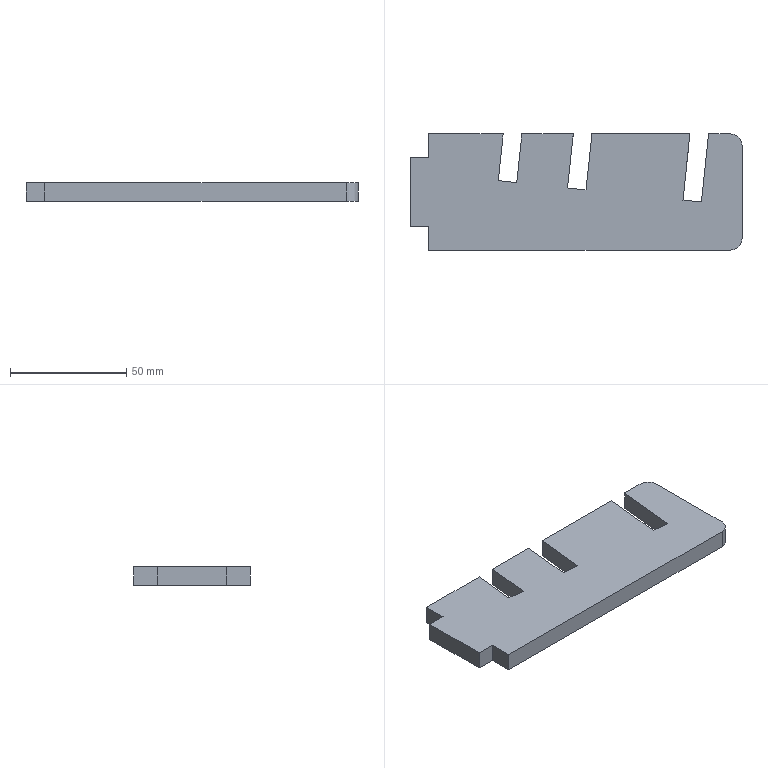Part | SolidWorks | features Fillet 1, FlatPattern 1, SMBaseFlange 1, SheetMetal 1 | 1 solid | 24 faces | box 143 x 50 x 8 mm | volume 51129 mm3 | plane 22 | cylinder 2 | commonest cylinder face diameters 10 x2
STEP:
#1=CARTESIAN_POINT('',(690.834,-177.819,0.));
#2=VERTEX_POINT('',#1);
#3=CARTESIAN_POINT('',(693.823,-149.341,0.));
#4=VERTEX_POINT('',#3);
#5=CARTESIAN_POINT('',(693.823,-149.341,0.));
#6=DIRECTION('',(0.1044,0.9945,0.));
#7=VECTOR('',#6,1000.);
#8=LINE('',#5,#7);
#9=EDGE_CURVE('',#2,#4,#8,.T.);
#10=ORIENTED_EDGE('',*,*,#9,.F.);
#11=CARTESIAN_POINT('',(690.834,-177.819,-8.));
#12=VERTEX_POINT('',#11);
#13=CARTESIAN_POINT('',(690.834,-177.819,-8.));
#14=DIRECTION('',(0.,0.,1.));
#15=VECTOR('',#14,1000.);
#16=LINE('',#13,#15);
#17=EDGE_CURVE('',#12,#2,#16,.T.);
#18=ORIENTED_EDGE('',*,*,#17,.F.);
#19=CARTESIAN_POINT('',(693.823,-149.341,-8.));
#20=VERTEX_POINT('',#19);
#21=CARTESIAN_POINT('',(693.823,-149.341,-8.));
#22=DIRECTION('',(0.1044,0.9945,0.));
#23=VECTOR('',#22,1000.);
#24=LINE('',#21,#23);
#25=EDGE_CURVE('',#12,#20,#24,.T.);
#26=ORIENTED_EDGE('',*,*,#25,.T.);
#27=CARTESIAN_POINT('',(693.823,-149.341,-8.));
#28=DIRECTION('',(0.,0.,1.));
#29=VECTOR('',#28,1000.);
#30=LINE('',#27,#29);
#31=EDGE_CURVE('',#20,#4,#30,.T.);
#32=ORIENTED_EDGE('',*,*,#31,.T.);
#33=EDGE_LOOP('',(#10,#18,#26,#32));
#34=FACE_OUTER_BOUND('',#33,.T.);
#35=CARTESIAN_POINT('',(693.823,-149.341,-8.));
#36=DIRECTION('',(0.9945,-0.1044,0.));
#37=DIRECTION('',(0.1044,0.9945,0.));
#38=AXIS2_PLACEMENT_3D('',#35,#36,#37);
#39=PLANE('',#38);
#40=ADVANCED_FACE('',(#34),#39,.T.);
#41=CARTESIAN_POINT('',(698.79,-178.654,0.));
#42=VERTEX_POINT('',#41);
#43=CARTESIAN_POINT('',(690.834,-177.819,0.));
#44=DIRECTION('',(-0.9945,0.1044,0.));
#45=VECTOR('',#44,1000.);
#46=LINE('',#43,#45);
#47=EDGE_CURVE('',#42,#2,#46,.T.);
#48=ORIENTED_EDGE('',*,*,#47,.F.);
#49=CARTESIAN_POINT('',(698.79,-178.654,-8.));
#50=VERTEX_POINT('',#49);
#51=CARTESIAN_POINT('',(698.79,-178.654,-8.));
#52=DIRECTION('',(0.,0.,1.));
#53=VECTOR('',#52,1000.);
#54=LINE('',#51,#53);
#55=EDGE_CURVE('',#50,#42,#54,.T.);
#56=ORIENTED_EDGE('',*,*,#55,.F.);
#57=CARTESIAN_POINT('',(690.834,-177.819,-8.));
#58=DIRECTION('',(-0.9945,0.1044,0.));
#59=VECTOR('',#58,1000.);
#60=LINE('',#57,#59);
#61=EDGE_CURVE('',#50,#12,#60,.T.);
#62=ORIENTED_EDGE('',*,*,#61,.T.);
#63=ORIENTED_EDGE('',*,*,#17,.T.);
#64=EDGE_LOOP('',(#48,#56,#62,#63));
#65=FACE_OUTER_BOUND('',#64,.T.);
#66=CARTESIAN_POINT('',(690.834,-177.819,-8.));
#67=DIRECTION('',(0.1044,0.9945,0.));
#68=DIRECTION('',(-0.9945,0.1044,0.));
#69=AXIS2_PLACEMENT_3D('',#66,#67,#68);
#70=PLANE('',#69);
#71=ADVANCED_FACE('',(#65),#70,.T.);
#72=CARTESIAN_POINT('',(701.867,-149.341,0.));
#73=VERTEX_POINT('',#72);
#74=CARTESIAN_POINT('',(698.79,-178.654,0.));
#75=DIRECTION('',(-0.1044,-0.9945,0.));
#76=VECTOR('',#75,1000.);
#77=LINE('',#74,#76);
#78=EDGE_CURVE('',#73,#42,#77,.T.);
#79=ORIENTED_EDGE('',*,*,#78,.F.);
#80=CARTESIAN_POINT('',(701.867,-149.341,-8.));
#81=VERTEX_POINT('',#80);
#82=CARTESIAN_POINT('',(701.867,-149.341,-8.));
#83=DIRECTION('',(0.,0.,1.));
#84=VECTOR('',#83,1000.);
#85=LINE('',#82,#84);
#86=EDGE_CURVE('',#81,#73,#85,.T.);
#87=ORIENTED_EDGE('',*,*,#86,.F.);
#88=CARTESIAN_POINT('',(698.79,-178.654,-8.));
#89=DIRECTION('',(-0.1044,-0.9945,0.));
#90=VECTOR('',#89,1000.);
#91=LINE('',#88,#90);
#92=EDGE_CURVE('',#81,#50,#91,.T.);
#93=ORIENTED_EDGE('',*,*,#92,.T.);
#94=ORIENTED_EDGE('',*,*,#55,.T.);
#95=EDGE_LOOP('',(#79,#87,#93,#94));
#96=FACE_OUTER_BOUND('',#95,.T.);
#97=CARTESIAN_POINT('',(698.79,-178.654,-8.));
#98=DIRECTION('',(-0.9945,0.1044,0.));
#99=DIRECTION('',(-0.1044,-0.9945,0.));
#100=AXIS2_PLACEMENT_3D('',#97,#98,#99);
#101=PLANE('',#100);
#102=ADVANCED_FACE('',(#96),#101,.T.);
#103=CARTESIAN_POINT('',(711.248,-149.341,0.));
#104=VERTEX_POINT('',#103);
#105=CARTESIAN_POINT('',(701.867,-149.341,0.));
#106=DIRECTION('',(-1.,0.,0.));
#107=VECTOR('',#106,1000.);
#108=LINE('',#105,#107);
#109=EDGE_CURVE('',#104,#73,#108,.T.);
#110=ORIENTED_EDGE('',*,*,#109,.F.);
#111=CARTESIAN_POINT('',(711.248,-149.341,-8.));
#112=VERTEX_POINT('',#111);
#113=CARTESIAN_POINT('',(711.248,-149.341,-8.));
#114=DIRECTION('',(0.,0.,-1.));
#115=VECTOR('',#114,1000.);
#116=LINE('',#113,#115);
#117=EDGE_CURVE('',#104,#112,#116,.T.);
#118=ORIENTED_EDGE('',*,*,#117,.T.);
#119=CARTESIAN_POINT('',(701.867,-149.341,-8.));
#120=DIRECTION('',(-1.,0.,0.));
#121=VECTOR('',#120,1000.);
#122=LINE('',#119,#121);
#123=EDGE_CURVE('',#112,#81,#122,.T.);
#124=ORIENTED_EDGE('',*,*,#123,.T.);
#125=ORIENTED_EDGE('',*,*,#86,.T.);
#126=EDGE_LOOP('',(#110,#118,#124,#125));
#127=FACE_OUTER_BOUND('',#126,.T.);
#128=CARTESIAN_POINT('',(701.867,-149.341,-8.));
#129=DIRECTION('',(0.,1.,0.));
#130=DIRECTION('',(0.,0.,1.));
#131=AXIS2_PLACEMENT_3D('',#128,#129,#130);
#132=PLANE('',#131);
#133=ADVANCED_FACE('',(#127),#132,.T.);
#134=CARTESIAN_POINT('',(716.248,-194.341,-8.));
#135=VERTEX_POINT('',#134);
#136=CARTESIAN_POINT('',(716.248,-154.341,-8.));
#137=VERTEX_POINT('',#136);
#138=CARTESIAN_POINT('',(716.248,-149.341,-8.));
#139=DIRECTION('',(0.,1.,0.));
#140=VECTOR('',#139,1000.);
#141=LINE('',#138,#140);
#142=EDGE_CURVE('',#135,#137,#141,.T.);
#143=ORIENTED_EDGE('',*,*,#142,.T.);
#144=CARTESIAN_POINT('',(716.248,-154.341,0.));
#145=VERTEX_POINT('',#144);
#146=CARTESIAN_POINT('',(716.248,-154.341,-8.));
#147=DIRECTION('',(0.,0.,1.));
#148=VECTOR('',#147,1000.);
#149=LINE('',#146,#148);
#150=EDGE_CURVE('',#137,#145,#149,.T.);
#151=ORIENTED_EDGE('',*,*,#150,.T.);
#152=CARTESIAN_POINT('',(716.248,-194.341,0.));
#153=VERTEX_POINT('',#152);
#154=CARTESIAN_POINT('',(716.248,-149.341,0.));
#155=DIRECTION('',(0.,1.,0.));
#156=VECTOR('',#155,1000.);
#157=LINE('',#154,#156);
#158=EDGE_CURVE('',#153,#145,#157,.T.);
#159=ORIENTED_EDGE('',*,*,#158,.F.);
#160=CARTESIAN_POINT('',(716.248,-194.341,-8.));
#161=DIRECTION('',(0.,0.,-1.));
#162=VECTOR('',#161,1000.);
#163=LINE('',#160,#162);
#164=EDGE_CURVE('',#153,#135,#163,.T.);
#165=ORIENTED_EDGE('',*,*,#164,.T.);
#166=EDGE_LOOP('',(#143,#151,#159,#165));
#167=FACE_OUTER_BOUND('',#166,.T.);
#168=CARTESIAN_POINT('',(716.248,-149.341,-8.));
#169=DIRECTION('',(1.,0.,0.));
#170=DIRECTION('',(0.,0.,-1.));
#171=AXIS2_PLACEMENT_3D('',#168,#169,#170);
#172=PLANE('',#171);
#173=ADVANCED_FACE('',(#167),#172,.T.);
#174=CARTESIAN_POINT('',(581.248,-199.341,-8.));
#175=VERTEX_POINT('',#174);
#176=CARTESIAN_POINT('',(711.248,-199.341,-8.));
#177=VERTEX_POINT('',#176);
#178=CARTESIAN_POINT('',(581.248,-199.341,-8.));
#179=DIRECTION('',(1.,0.,0.));
#180=VECTOR('',#179,1000.);
#181=LINE('',#178,#180);
#182=EDGE_CURVE('',#175,#177,#181,.T.);
#183=ORIENTED_EDGE('',*,*,#182,.T.);
#184=CARTESIAN_POINT('',(711.248,-199.341,0.));
#185=VERTEX_POINT('',#184);
#186=CARTESIAN_POINT('',(711.248,-199.341,-8.));
#187=DIRECTION('',(0.,0.,1.));
#188=VECTOR('',#187,1000.);
#189=LINE('',#186,#188);
#190=EDGE_CURVE('',#177,#185,#189,.T.);
#191=ORIENTED_EDGE('',*,*,#190,.T.);
#192=CARTESIAN_POINT('',(581.248,-199.341,0.));
#193=VERTEX_POINT('',#192);
#194=CARTESIAN_POINT('',(581.248,-199.341,0.));
#195=DIRECTION('',(1.,0.,0.));
#196=VECTOR('',#195,1000.);
#197=LINE('',#194,#196);
#198=EDGE_CURVE('',#193,#185,#197,.T.);
#199=ORIENTED_EDGE('',*,*,#198,.F.);
#200=CARTESIAN_POINT('',(581.248,-199.341,-8.));
#201=DIRECTION('',(0.,0.,1.));
#202=VECTOR('',#201,1000.);
#203=LINE('',#200,#202);
#204=EDGE_CURVE('',#175,#193,#203,.T.);
#205=ORIENTED_EDGE('',*,*,#204,.F.);
#206=EDGE_LOOP('',(#183,#191,#199,#205));
#207=FACE_OUTER_BOUND('',#206,.T.);
#208=CARTESIAN_POINT('',(581.248,-199.341,-8.));
#209=DIRECTION('',(0.,-1.,0.));
#210=DIRECTION('',(0.,0.,-1.));
#211=AXIS2_PLACEMENT_3D('',#208,#209,#210);
#212=PLANE('',#211);
#213=ADVANCED_FACE('',(#207),#212,.T.);
#214=CARTESIAN_POINT('',(581.248,-189.341,0.));
#215=VERTEX_POINT('',#214);
#216=CARTESIAN_POINT('',(581.248,-189.341,0.));
#217=DIRECTION('',(0.,-1.,0.));
#218=VECTOR('',#217,1000.);
#219=LINE('',#216,#218);
#220=EDGE_CURVE('',#215,#193,#219,.T.);
#221=ORIENTED_EDGE('',*,*,#220,.F.);
#222=CARTESIAN_POINT('',(581.248,-189.341,-8.));
#223=VERTEX_POINT('',#222);
#224=CARTESIAN_POINT('',(581.248,-189.341,-8.));
#225=DIRECTION('',(0.,0.,1.));
#226=VECTOR('',#225,1000.);
#227=LINE('',#224,#226);
#228=EDGE_CURVE('',#223,#215,#227,.T.);
#229=ORIENTED_EDGE('',*,*,#228,.F.);
#230=CARTESIAN_POINT('',(581.248,-189.341,-8.));
#231=DIRECTION('',(0.,-1.,0.));
#232=VECTOR('',#231,1000.);
#233=LINE('',#230,#232);
#234=EDGE_CURVE('',#223,#175,#233,.T.);
#235=ORIENTED_EDGE('',*,*,#234,.T.);
#236=ORIENTED_EDGE('',*,*,#204,.T.);
#237=EDGE_LOOP('',(#221,#229,#235,#236));
#238=FACE_OUTER_BOUND('',#237,.T.);
#239=CARTESIAN_POINT('',(581.248,-189.341,-8.));
#240=DIRECTION('',(-1.,0.,0.));
#241=DIRECTION('',(0.,0.,1.));
#242=AXIS2_PLACEMENT_3D('',#239,#240,#241);
#243=PLANE('',#242);
#244=ADVANCED_FACE('',(#238),#243,.T.);
#245=CARTESIAN_POINT('',(573.248,-189.341,0.));
#246=VERTEX_POINT('',#245);
#247=CARTESIAN_POINT('',(573.248,-189.341,0.));
#248=DIRECTION('',(1.,0.,0.));
#249=VECTOR('',#248,1000.);
#250=LINE('',#247,#249);
#251=EDGE_CURVE('',#246,#215,#250,.T.);
#252=ORIENTED_EDGE('',*,*,#251,.F.);
#253=CARTESIAN_POINT('',(573.248,-189.341,-8.));
#254=VERTEX_POINT('',#253);
#255=CARTESIAN_POINT('',(573.248,-189.341,-8.));
#256=DIRECTION('',(0.,0.,1.));
#257=VECTOR('',#256,1000.);
#258=LINE('',#255,#257);
#259=EDGE_CURVE('',#254,#246,#258,.T.);
#260=ORIENTED_EDGE('',*,*,#259,.F.);
#261=CARTESIAN_POINT('',(573.248,-189.341,-8.));
#262=DIRECTION('',(1.,0.,0.));
#263=VECTOR('',#262,1000.);
#264=LINE('',#261,#263);
#265=EDGE_CURVE('',#254,#223,#264,.T.);
#266=ORIENTED_EDGE('',*,*,#265,.T.);
#267=ORIENTED_EDGE('',*,*,#228,.T.);
#268=EDGE_LOOP('',(#252,#260,#266,#267));
#269=FACE_OUTER_BOUND('',#268,.T.);
#270=CARTESIAN_POINT('',(573.248,-189.341,-8.));
#271=DIRECTION('',(0.,-1.,0.));
#272=DIRECTION('',(0.,0.,-1.));
#273=AXIS2_PLACEMENT_3D('',#270,#271,#272);
#274=PLANE('',#273);
#275=ADVANCED_FACE('',(#269),#274,.T.);
#276=CARTESIAN_POINT('',(573.248,-159.341,0.));
#277=VERTEX_POINT('',#276);
#278=CARTESIAN_POINT('',(573.248,-159.341,0.));
#279=DIRECTION('',(0.,-1.,0.));
#280=VECTOR('',#279,1000.);
#281=LINE('',#278,#280);
#282=EDGE_CURVE('',#277,#246,#281,.T.);
#283=ORIENTED_EDGE('',*,*,#282,.F.);
#284=CARTESIAN_POINT('',(573.248,-159.341,-8.));
#285=VERTEX_POINT('',#284);
#286=CARTESIAN_POINT('',(573.248,-159.341,-8.));
#287=DIRECTION('',(0.,0.,1.));
#288=VECTOR('',#287,1000.);
#289=LINE('',#286,#288);
#290=EDGE_CURVE('',#285,#277,#289,.T.);
#291=ORIENTED_EDGE('',*,*,#290,.F.);
#292=CARTESIAN_POINT('',(573.248,-159.341,-8.));
#293=DIRECTION('',(0.,-1.,0.));
#294=VECTOR('',#293,1000.);
#295=LINE('',#292,#294);
#296=EDGE_CURVE('',#285,#254,#295,.T.);
#297=ORIENTED_EDGE('',*,*,#296,.T.);
#298=ORIENTED_EDGE('',*,*,#259,.T.);
#299=EDGE_LOOP('',(#283,#291,#297,#298));
#300=FACE_OUTER_BOUND('',#299,.T.);
#301=CARTESIAN_POINT('',(573.248,-159.341,-8.));
#302=DIRECTION('',(-1.,0.,0.));
#303=DIRECTION('',(0.,0.,1.));
#304=AXIS2_PLACEMENT_3D('',#301,#302,#303);
#305=PLANE('',#304);
#306=ADVANCED_FACE('',(#300),#305,.T.);
#307=CARTESIAN_POINT('',(581.248,-159.341,0.));
#308=VERTEX_POINT('',#307);
#309=CARTESIAN_POINT('',(581.248,-159.341,0.));
#310=DIRECTION('',(-1.,0.,0.));
#311=VECTOR('',#310,1000.);
#312=LINE('',#309,#311);
#313=EDGE_CURVE('',#308,#277,#312,.T.);
#314=ORIENTED_EDGE('',*,*,#313,.F.);
#315=CARTESIAN_POINT('',(581.248,-159.341,-8.));
#316=VERTEX_POINT('',#315);
#317=CARTESIAN_POINT('',(581.248,-159.341,-8.));
#318=DIRECTION('',(0.,0.,1.));
#319=VECTOR('',#318,1000.);
#320=LINE('',#317,#319);
#321=EDGE_CURVE('',#316,#308,#320,.T.);
#322=ORIENTED_EDGE('',*,*,#321,.F.);
#323=CARTESIAN_POINT('',(581.248,-159.341,-8.));
#324=DIRECTION('',(-1.,0.,0.));
#325=VECTOR('',#324,1000.);
#326=LINE('',#323,#325);
#327=EDGE_CURVE('',#316,#285,#326,.T.);
#328=ORIENTED_EDGE('',*,*,#327,.T.);
#329=ORIENTED_EDGE('',*,*,#290,.T.);
#330=EDGE_LOOP('',(#314,#322,#328,#329));
#331=FACE_OUTER_BOUND('',#330,.T.);
#332=CARTESIAN_POINT('',(581.248,-159.341,-8.));
#333=DIRECTION('',(0.,1.,0.));
#334=DIRECTION('',(0.,0.,1.));
#335=AXIS2_PLACEMENT_3D('',#332,#333,#334);
#336=PLANE('',#335);
#337=ADVANCED_FACE('',(#331),#336,.T.);
#338=CARTESIAN_POINT('',(581.248,-149.341,0.));
#339=VERTEX_POINT('',#338);
#340=CARTESIAN_POINT('',(581.248,-149.341,0.));
#341=DIRECTION('',(0.,-1.,0.));
#342=VECTOR('',#341,1000.);
#343=LINE('',#340,#342);
#344=EDGE_CURVE('',#339,#308,#343,.T.);
#345=ORIENTED_EDGE('',*,*,#344,.F.);
#346=CARTESIAN_POINT('',(581.248,-149.341,-8.));
#347=VERTEX_POINT('',#346);
#348=CARTESIAN_POINT('',(581.248,-149.341,-8.));
#349=DIRECTION('',(0.,0.,1.));
#350=VECTOR('',#349,1000.);
#351=LINE('',#348,#350);
#352=EDGE_CURVE('',#347,#339,#351,.T.);
#353=ORIENTED_EDGE('',*,*,#352,.F.);
#354=CARTESIAN_POINT('',(581.248,-149.341,-8.));
#355=DIRECTION('',(0.,-1.,0.));
#356=VECTOR('',#355,1000.);
#357=LINE('',#354,#356);
#358=EDGE_CURVE('',#347,#316,#357,.T.);
#359=ORIENTED_EDGE('',*,*,#358,.T.);
#360=ORIENTED_EDGE('',*,*,#321,.T.);
#361=EDGE_LOOP('',(#345,#353,#359,#360));
#362=FACE_OUTER_BOUND('',#361,.T.);
#363=CARTESIAN_POINT('',(581.248,-149.341,-8.));
#364=DIRECTION('',(-1.,0.,0.));
#365=DIRECTION('',(0.,0.,1.));
#366=AXIS2_PLACEMENT_3D('',#363,#364,#365);
#367=PLANE('',#366);
#368=ADVANCED_FACE('',(#362),#367,.T.);
#369=CARTESIAN_POINT('',(613.384,-149.341,0.));
#370=VERTEX_POINT('',#369);
#371=CARTESIAN_POINT('',(581.248,-149.341,0.));
#372=DIRECTION('',(-1.,0.,0.));
#373=VECTOR('',#372,1000.);
#374=LINE('',#371,#373);
#375=EDGE_CURVE('',#370,#339,#374,.T.);
#376=ORIENTED_EDGE('',*,*,#375,.F.);
#377=CARTESIAN_POINT('',(613.384,-149.341,-8.));
#378=VERTEX_POINT('',#377);
#379=CARTESIAN_POINT('',(613.384,-149.341,-8.));
#380=DIRECTION('',(0.,0.,1.));
#381=VECTOR('',#380,1000.);
#382=LINE('',#379,#381);
#383=EDGE_CURVE('',#378,#370,#382,.T.);
#384=ORIENTED_EDGE('',*,*,#383,.F.);
#385=CARTESIAN_POINT('',(581.248,-149.341,-8.));
#386=DIRECTION('',(-1.,0.,0.));
#387=VECTOR('',#386,1000.);
#388=LINE('',#385,#387);
#389=EDGE_CURVE('',#378,#347,#388,.T.);
#390=ORIENTED_EDGE('',*,*,#389,.T.);
#391=ORIENTED_EDGE('',*,*,#352,.T.);
#392=EDGE_LOOP('',(#376,#384,#390,#391));
#393=FACE_OUTER_BOUND('',#392,.T.);
#394=CARTESIAN_POINT('',(581.248,-149.341,-8.));
#395=DIRECTION('',(0.,1.,0.));
#396=DIRECTION('',(0.,0.,1.));
#397=AXIS2_PLACEMENT_3D('',#394,#395,#396);
#398=PLANE('',#397);
#399=ADVANCED_FACE('',(#393),#398,.T.);
#400=CARTESIAN_POINT('',(611.271,-169.465,0.));
#401=VERTEX_POINT('',#400);
#402=CARTESIAN_POINT('',(611.271,-169.465,0.));
#403=DIRECTION('',(0.1044,0.9945,0.));
#404=VECTOR('',#403,1000.);
#405=LINE('',#402,#404);
#406=EDGE_CURVE('',#401,#370,#405,.T.);
#407=ORIENTED_EDGE('',*,*,#406,.F.);
#408=CARTESIAN_POINT('',(611.271,-169.465,-8.));
#409=VERTEX_POINT('',#408);
#410=CARTESIAN_POINT('',(611.271,-169.465,-8.));
#411=DIRECTION('',(0.,0.,1.));
#412=VECTOR('',#411,1000.);
#413=LINE('',#410,#412);
#414=EDGE_CURVE('',#409,#401,#413,.T.);
#415=ORIENTED_EDGE('',*,*,#414,.F.);
#416=CARTESIAN_POINT('',(611.271,-169.465,-8.));
#417=DIRECTION('',(0.1044,0.9945,0.));
#418=VECTOR('',#417,1000.);
#419=LINE('',#416,#418);
#420=EDGE_CURVE('',#409,#378,#419,.T.);
#421=ORIENTED_EDGE('',*,*,#420,.T.);
#422=ORIENTED_EDGE('',*,*,#383,.T.);
#423=EDGE_LOOP('',(#407,#415,#421,#422));
#424=FACE_OUTER_BOUND('',#423,.T.);
#425=CARTESIAN_POINT('',(611.271,-169.465,-8.));
#426=DIRECTION('',(0.9945,-0.1044,0.));
#427=DIRECTION('',(0.1044,0.9945,0.));
#428=AXIS2_PLACEMENT_3D('',#425,#426,#427);
#429=PLANE('',#428);
#430=ADVANCED_FACE('',(#424),#429,.T.);
#431=CARTESIAN_POINT('',(619.227,-170.301,0.));
#432=VERTEX_POINT('',#431);
#433=CARTESIAN_POINT('',(611.271,-169.465,0.));
#434=DIRECTION('',(-0.9945,0.1044,0.));
#435=VECTOR('',#434,1000.);
#436=LINE('',#433,#435);
#437=EDGE_CURVE('',#432,#401,#436,.T.);
#438=ORIENTED_EDGE('',*,*,#437,.F.);
#439=CARTESIAN_POINT('',(619.227,-170.301,-8.));
#440=VERTEX_POINT('',#439);
#441=CARTESIAN_POINT('',(619.227,-170.301,-8.));
#442=DIRECTION('',(0.,0.,1.));
#443=VECTOR('',#442,1000.);
#444=LINE('',#441,#443);
#445=EDGE_CURVE('',#440,#432,#444,.T.);
#446=ORIENTED_EDGE('',*,*,#445,.F.);
#447=CARTESIAN_POINT('',(611.271,-169.465,-8.));
#448=DIRECTION('',(-0.9945,0.1044,0.));
#449=VECTOR('',#448,1000.);
#450=LINE('',#447,#449);
#451=EDGE_CURVE('',#440,#409,#450,.T.);
#452=ORIENTED_EDGE('',*,*,#451,.T.);
#453=ORIENTED_EDGE('',*,*,#414,.T.);
#454=EDGE_LOOP('',(#438,#446,#452,#453));
#455=FACE_OUTER_BOUND('',#454,.T.);
#456=CARTESIAN_POINT('',(611.271,-169.465,-8.));
#457=DIRECTION('',(0.1044,0.9945,0.));
#458=DIRECTION('',(-0.9945,0.1044,0.));
#459=AXIS2_PLACEMENT_3D('',#456,#457,#458);
#460=PLANE('',#459);
#461=ADVANCED_FACE('',(#455),#460,.T.);
#462=CARTESIAN_POINT('',(621.428,-149.341,0.));
#463=VERTEX_POINT('',#462);
#464=CARTESIAN_POINT('',(619.227,-170.301,0.));
#465=DIRECTION('',(-0.1044,-0.9945,0.));
#466=VECTOR('',#465,1000.);
#467=LINE('',#464,#466);
#468=EDGE_CURVE('',#463,#432,#467,.T.);
#469=ORIENTED_EDGE('',*,*,#468,.F.);
#470=CARTESIAN_POINT('',(621.428,-149.341,-8.));
#471=VERTEX_POINT('',#470);
#472=CARTESIAN_POINT('',(621.428,-149.341,-8.));
#473=DIRECTION('',(0.,0.,1.));
#474=VECTOR('',#473,1000.);
#475=LINE('',#472,#474);
#476=EDGE_CURVE('',#471,#463,#475,.T.);
#477=ORIENTED_EDGE('',*,*,#476,.F.);
#478=CARTESIAN_POINT('',(619.227,-170.301,-8.));
#479=DIRECTION('',(-0.1044,-0.9945,0.));
#480=VECTOR('',#479,1000.);
#481=LINE('',#478,#480);
#482=EDGE_CURVE('',#471,#440,#481,.T.);
#483=ORIENTED_EDGE('',*,*,#482,.T.);
#484=ORIENTED_EDGE('',*,*,#445,.T.);
#485=EDGE_LOOP('',(#469,#477,#483,#484));
#486=FACE_OUTER_BOUND('',#485,.T.);
#487=CARTESIAN_POINT('',(619.227,-170.301,-8.));
#488=DIRECTION('',(-0.9945,0.1044,0.));
#489=DIRECTION('',(-0.1044,-0.9945,0.));
#490=AXIS2_PLACEMENT_3D('',#487,#488,#489);
#491=PLANE('',#490);
#492=ADVANCED_FACE('',(#486),#491,.T.);
#493=CARTESIAN_POINT('',(643.549,-149.341,0.));
#494=VERTEX_POINT('',#493);
#495=CARTESIAN_POINT('',(621.428,-149.341,0.));
#496=DIRECTION('',(-1.,0.,0.));
#497=VECTOR('',#496,1000.);
#498=LINE('',#495,#497);
#499=EDGE_CURVE('',#494,#463,#498,.T.);
#500=ORIENTED_EDGE('',*,*,#499,.F.);
#501=CARTESIAN_POINT('',(643.549,-149.341,-8.));
#502=VERTEX_POINT('',#501);
#503=CARTESIAN_POINT('',(643.549,-149.341,-8.));
#504=DIRECTION('',(0.,0.,1.));
#505=VECTOR('',#504,1000.);
#506=LINE('',#503,#505);
#507=EDGE_CURVE('',#502,#494,#506,.T.);
#508=ORIENTED_EDGE('',*,*,#507,.F.);
#509=CARTESIAN_POINT('',(621.428,-149.341,-8.));
#510=DIRECTION('',(-1.,0.,0.));
#511=VECTOR('',#510,1000.);
#512=LINE('',#509,#511);
#513=EDGE_CURVE('',#502,#471,#512,.T.);
#514=ORIENTED_EDGE('',*,*,#513,.T.);
#515=ORIENTED_EDGE('',*,*,#476,.T.);
#516=EDGE_LOOP('',(#500,#508,#514,#515));
#517=FACE_OUTER_BOUND('',#516,.T.);
#518=CARTESIAN_POINT('',(621.428,-149.341,-8.));
#519=DIRECTION('',(0.,1.,0.));
#520=DIRECTION('',(0.,0.,1.));
#521=AXIS2_PLACEMENT_3D('',#518,#519,#520);
#522=PLANE('',#521);
#523=ADVANCED_FACE('',(#517),#522,.T.);
#524=CARTESIAN_POINT('',(641.107,-172.598,0.));
#525=VERTEX_POINT('',#524);
#526=CARTESIAN_POINT('',(641.107,-172.598,0.));
#527=DIRECTION('',(0.1044,0.9945,0.));
#528=VECTOR('',#527,1000.);
#529=LINE('',#526,#528);
#530=EDGE_CURVE('',#525,#494,#529,.T.);
#531=ORIENTED_EDGE('',*,*,#530,.F.);
#532=CARTESIAN_POINT('',(641.107,-172.598,-8.));
#533=VERTEX_POINT('',#532);
#534=CARTESIAN_POINT('',(641.107,-172.598,-8.));
#535=DIRECTION('',(0.,0.,1.));
#536=VECTOR('',#535,1000.);
#537=LINE('',#534,#536);
#538=EDGE_CURVE('',#533,#525,#537,.T.);
#539=ORIENTED_EDGE('',*,*,#538,.F.);
#540=CARTESIAN_POINT('',(641.107,-172.598,-8.));
#541=DIRECTION('',(0.1044,0.9945,0.));
#542=VECTOR('',#541,1000.);
#543=LINE('',#540,#542);
#544=EDGE_CURVE('',#533,#502,#543,.T.);
#545=ORIENTED_EDGE('',*,*,#544,.T.);
#546=ORIENTED_EDGE('',*,*,#507,.T.);
#547=EDGE_LOOP('',(#531,#539,#545,#546));
#548=FACE_OUTER_BOUND('',#547,.T.);
#549=CARTESIAN_POINT('',(641.107,-172.598,-8.));
#550=DIRECTION('',(0.9945,-0.1044,0.));
#551=DIRECTION('',(0.1044,0.9945,0.));
#552=AXIS2_PLACEMENT_3D('',#549,#550,#551);
#553=PLANE('',#552);
#554=ADVANCED_FACE('',(#548),#553,.T.);
#555=CARTESIAN_POINT('',(649.063,-173.433,0.));
#556=VERTEX_POINT('',#555);
#557=CARTESIAN_POINT('',(649.063,-173.433,0.));
#558=DIRECTION('',(-0.9945,0.1044,0.));
#559=VECTOR('',#558,1000.);
#560=LINE('',#557,#559);
#561=EDGE_CURVE('',#556,#525,#560,.T.);
#562=ORIENTED_EDGE('',*,*,#561,.F.);
#563=CARTESIAN_POINT('',(649.063,-173.433,-8.));
#564=VERTEX_POINT('',#563);
#565=CARTESIAN_POINT('',(649.063,-173.433,-8.));
#566=DIRECTION('',(0.,0.,1.));
#567=VECTOR('',#566,1000.);
#568=LINE('',#565,#567);
#569=EDGE_CURVE('',#564,#556,#568,.T.);
#570=ORIENTED_EDGE('',*,*,#569,.F.);
#571=CARTESIAN_POINT('',(649.063,-173.433,-8.));
#572=DIRECTION('',(-0.9945,0.1044,0.));
#573=VECTOR('',#572,1000.);
#574=LINE('',#571,#573);
#575=EDGE_CURVE('',#564,#533,#574,.T.);
#576=ORIENTED_EDGE('',*,*,#575,.T.);
#577=ORIENTED_EDGE('',*,*,#538,.T.);
#578=EDGE_LOOP('',(#562,#570,#576,#577));
#579=FACE_OUTER_BOUND('',#578,.T.);
#580=CARTESIAN_POINT('',(649.063,-173.433,-8.));
#581=DIRECTION('',(0.1044,0.9945,0.));
#582=DIRECTION('',(-0.9945,0.1044,0.));
#583=AXIS2_PLACEMENT_3D('',#580,#581,#582);
#584=PLANE('',#583);
#585=ADVANCED_FACE('',(#579),#584,.T.);
#586=CARTESIAN_POINT('',(651.593,-149.341,0.));
#587=VERTEX_POINT('',#586);
#588=CARTESIAN_POINT('',(649.063,-173.433,0.));
#589=DIRECTION('',(-0.1044,-0.9945,0.));
#590=VECTOR('',#589,1000.);
#591=LINE('',#588,#590);
#592=EDGE_CURVE('',#587,#556,#591,.T.);
#593=ORIENTED_EDGE('',*,*,#592,.F.);
#594=CARTESIAN_POINT('',(651.593,-149.341,-8.));
#595=VERTEX_POINT('',#594);
#596=CARTESIAN_POINT('',(651.593,-149.341,-8.));
#597=DIRECTION('',(0.,0.,1.));
#598=VECTOR('',#597,1000.);
#599=LINE('',#596,#598);
#600=EDGE_CURVE('',#595,#587,#599,.T.);
#601=ORIENTED_EDGE('',*,*,#600,.F.);
#602=CARTESIAN_POINT('',(649.063,-173.433,-8.));
#603=DIRECTION('',(-0.1044,-0.9945,0.));
#604=VECTOR('',#603,1000.);
#605=LINE('',#602,#604);
#606=EDGE_CURVE('',#595,#564,#605,.T.);
#607=ORIENTED_EDGE('',*,*,#606,.T.);
#608=ORIENTED_EDGE('',*,*,#569,.T.);
#609=EDGE_LOOP('',(#593,#601,#607,#608));
#610=FACE_OUTER_BOUND('',#609,.T.);
#611=CARTESIAN_POINT('',(649.063,-173.433,-8.));
#612=DIRECTION('',(-0.9945,0.1044,0.));
#613=DIRECTION('',(-0.1044,-0.9945,0.));
#614=AXIS2_PLACEMENT_3D('',#611,#612,#613);
#615=PLANE('',#614);
#616=ADVANCED_FACE('',(#610),#615,.T.);
#617=CARTESIAN_POINT('',(651.593,-149.341,0.));
#618=DIRECTION('',(-1.,0.,0.));
#619=VECTOR('',#618,1000.);
#620=LINE('',#617,#619);
#621=EDGE_CURVE('',#4,#587,#620,.T.);
#622=ORIENTED_EDGE('',*,*,#621,.F.);
#623=ORIENTED_EDGE('',*,*,#31,.F.);
#624=CARTESIAN_POINT('',(651.593,-149.341,-8.));
#625=DIRECTION('',(-1.,0.,0.));
#626=VECTOR('',#625,1000.);
#627=LINE('',#624,#626);
#628=EDGE_CURVE('',#20,#595,#627,.T.);
#629=ORIENTED_EDGE('',*,*,#628,.T.);
#630=ORIENTED_EDGE('',*,*,#600,.T.);
#631=EDGE_LOOP('',(#622,#623,#629,#630));
#632=FACE_OUTER_BOUND('',#631,.T.);
#633=CARTESIAN_POINT('',(651.593,-149.341,-8.));
#634=DIRECTION('',(0.,1.,0.));
#635=DIRECTION('',(0.,0.,1.));
#636=AXIS2_PLACEMENT_3D('',#633,#634,#635);
#637=PLANE('',#636);
#638=ADVANCED_FACE('',(#632),#637,.T.);
#639=ORIENTED_EDGE('',*,*,#123,.F.);
#640=CARTESIAN_POINT('',(711.248,-154.341,-8.));
#641=DIRECTION('',(0.,0.,-1.));
#642=DIRECTION('',(1.,0.,0.));
#643=AXIS2_PLACEMENT_3D('',#640,#641,#642);
#644=CIRCLE('',#643,5.);
#645=EDGE_CURVE('',#112,#137,#644,.T.);
#646=ORIENTED_EDGE('',*,*,#645,.T.);
#647=ORIENTED_EDGE('',*,*,#142,.F.);
#648=CARTESIAN_POINT('',(711.248,-194.341,-8.));
#649=DIRECTION('',(0.,0.,-1.));
#650=DIRECTION('',(1.,0.,0.));
#651=AXIS2_PLACEMENT_3D('',#648,#649,#650);
#652=CIRCLE('',#651,5.);
#653=EDGE_CURVE('',#135,#177,#652,.T.);
#654=ORIENTED_EDGE('',*,*,#653,.T.);
#655=ORIENTED_EDGE('',*,*,#182,.F.);
#656=ORIENTED_EDGE('',*,*,#234,.F.);
#657=ORIENTED_EDGE('',*,*,#265,.F.);
#658=ORIENTED_EDGE('',*,*,#296,.F.);
#659=ORIENTED_EDGE('',*,*,#327,.F.);
#660=ORIENTED_EDGE('',*,*,#358,.F.);
#661=ORIENTED_EDGE('',*,*,#389,.F.);
#662=ORIENTED_EDGE('',*,*,#420,.F.);
#663=ORIENTED_EDGE('',*,*,#451,.F.);
#664=ORIENTED_EDGE('',*,*,#482,.F.);
#665=ORIENTED_EDGE('',*,*,#513,.F.);
#666=ORIENTED_EDGE('',*,*,#544,.F.);
#667=ORIENTED_EDGE('',*,*,#575,.F.);
#668=ORIENTED_EDGE('',*,*,#606,.F.);
#669=ORIENTED_EDGE('',*,*,#628,.F.);
#670=ORIENTED_EDGE('',*,*,#25,.F.);
#671=ORIENTED_EDGE('',*,*,#61,.F.);
#672=ORIENTED_EDGE('',*,*,#92,.F.);
#673=EDGE_LOOP('',(#639,#646,#647,#654,#655,#656,#657,#658,#659,#660,#661,#662,#663,#664,#665,#666,#667,#668,#669,#670,#671,#672));
#674=FACE_OUTER_BOUND('',#673,.T.);
#675=CARTESIAN_POINT('',(0.,0.,-8.));
#676=DIRECTION('',(0.,0.,1.));
#677=DIRECTION('',(1.,0.,0.));
#678=AXIS2_PLACEMENT_3D('',#675,#676,#677);
#679=PLANE('',#678);
#680=ADVANCED_FACE('',(#674),#679,.F.);
#681=ORIENTED_EDGE('',*,*,#158,.T.);
#682=CARTESIAN_POINT('',(711.248,-154.341,0.));
#683=DIRECTION('',(0.,0.,1.));
#684=DIRECTION('',(1.,0.,0.));
#685=AXIS2_PLACEMENT_3D('',#682,#683,#684);
#686=CIRCLE('',#685,5.);
#687=EDGE_CURVE('',#145,#104,#686,.T.);
#688=ORIENTED_EDGE('',*,*,#687,.T.);
#689=ORIENTED_EDGE('',*,*,#109,.T.);
#690=ORIENTED_EDGE('',*,*,#78,.T.);
#691=ORIENTED_EDGE('',*,*,#47,.T.);
#692=ORIENTED_EDGE('',*,*,#9,.T.);
#693=ORIENTED_EDGE('',*,*,#621,.T.);
#694=ORIENTED_EDGE('',*,*,#592,.T.);
#695=ORIENTED_EDGE('',*,*,#561,.T.);
#696=ORIENTED_EDGE('',*,*,#530,.T.);
#697=ORIENTED_EDGE('',*,*,#499,.T.);
#698=ORIENTED_EDGE('',*,*,#468,.T.);
#699=ORIENTED_EDGE('',*,*,#437,.T.);
#700=ORIENTED_EDGE('',*,*,#406,.T.);
#701=ORIENTED_EDGE('',*,*,#375,.T.);
#702=ORIENTED_EDGE('',*,*,#344,.T.);
#703=ORIENTED_EDGE('',*,*,#313,.T.);
#704=ORIENTED_EDGE('',*,*,#282,.T.);
#705=ORIENTED_EDGE('',*,*,#251,.T.);
#706=ORIENTED_EDGE('',*,*,#220,.T.);
#707=ORIENTED_EDGE('',*,*,#198,.T.);
#708=CARTESIAN_POINT('',(711.248,-194.341,0.));
#709=DIRECTION('',(0.,0.,1.));
#710=DIRECTION('',(1.,0.,0.));
#711=AXIS2_PLACEMENT_3D('',#708,#709,#710);
#712=CIRCLE('',#711,5.);
#713=EDGE_CURVE('',#185,#153,#712,.T.);
#714=ORIENTED_EDGE('',*,*,#713,.T.);
#715=EDGE_LOOP('',(#681,#688,#689,#690,#691,#692,#693,#694,#695,#696,#697,#698,#699,#700,#701,#702,#703,#704,#705,#706,#707,#714));
#716=FACE_OUTER_BOUND('',#715,.T.);
#717=CARTESIAN_POINT('',(0.,0.,0.));
#718=DIRECTION('',(0.,0.,1.));
#719=DIRECTION('',(1.,0.,0.));
#720=AXIS2_PLACEMENT_3D('',#717,#718,#719);
#721=PLANE('',#720);
#722=ADVANCED_FACE('',(#716),#721,.T.);
#723=ORIENTED_EDGE('',*,*,#645,.F.);
#724=ORIENTED_EDGE('',*,*,#117,.F.);
#725=ORIENTED_EDGE('',*,*,#687,.F.);
#726=ORIENTED_EDGE('',*,*,#150,.F.);
#727=EDGE_LOOP('',(#723,#724,#725,#726));
#728=FACE_OUTER_BOUND('',#727,.T.);
#729=CARTESIAN_POINT('',(711.248,-154.341,-8.));
#730=DIRECTION('',(0.,0.,1.));
#731=DIRECTION('',(1.,0.,0.));
#732=AXIS2_PLACEMENT_3D('',#729,#730,#731);
#733=CYLINDRICAL_SURFACE('',#732,5.);
#734=ADVANCED_FACE('',(#728),#733,.T.);
#735=ORIENTED_EDGE('',*,*,#653,.F.);
#736=ORIENTED_EDGE('',*,*,#164,.F.);
#737=ORIENTED_EDGE('',*,*,#713,.F.);
#738=ORIENTED_EDGE('',*,*,#190,.F.);
#739=EDGE_LOOP('',(#735,#736,#737,#738));
#740=FACE_OUTER_BOUND('',#739,.T.);
#741=CARTESIAN_POINT('',(711.248,-194.341,-8.));
#742=DIRECTION('',(0.,0.,1.));
#743=DIRECTION('',(1.,0.,0.));
#744=AXIS2_PLACEMENT_3D('',#741,#742,#743);
#745=CYLINDRICAL_SURFACE('',#744,5.);
#746=ADVANCED_FACE('',(#740),#745,.T.);
#747=CLOSED_SHELL('',(#40,#71,#102,#133,#173,#213,#244,#275,#306,#337,#368,#399,#430,#461,#492,#523,#554,#585,#616,#638,#680,#722,#734,#746));
#748=MANIFOLD_SOLID_BREP('',#747);
#749=CARTESIAN_POINT('',(0.,0.,0.));
#750=DIRECTION('',(0.,0.,1.));
#751=DIRECTION('',(1.,0.,0.));
#752=AXIS2_PLACEMENT_3D('',#749,#750,#751);
#753=(LENGTH_UNIT()NAMED_UNIT(*)SI_UNIT(.MILLI.,.METRE.));
#754=UNCERTAINTY_MEASURE_WITH_UNIT(LENGTH_MEASURE(0.00001),#753,'','');
#755=(NAMED_UNIT(*)PLANE_ANGLE_UNIT()SI_UNIT($,.RADIAN.));
#756=(NAMED_UNIT(*)SI_UNIT($,.STERADIAN.)SOLID_ANGLE_UNIT());
#757=(GEOMETRIC_REPRESENTATION_CONTEXT(3)GLOBAL_UNCERTAINTY_ASSIGNED_CONTEXT((#754))GLOBAL_UNIT_ASSIGNED_CONTEXT((#753,#755,#756))REPRESENTATION_CONTEXT('',''));
#758=ADVANCED_BREP_SHAPE_REPRESENTATION('',(#748,#752),#757);